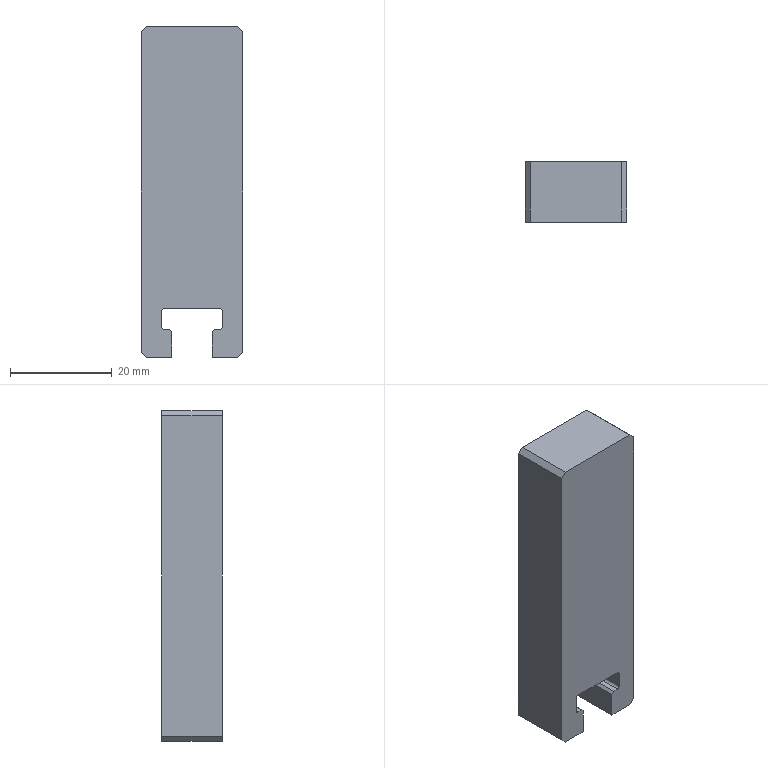Part | STEP file | PN_0026 | 1 solid | 40 faces | box 20 x 12 x 65 mm | volume 14321 mm3 | plane 20 | cylinder 12 | cone 8 | commonest cylinder face diameters 1 x4 2.5 x4 3 x4